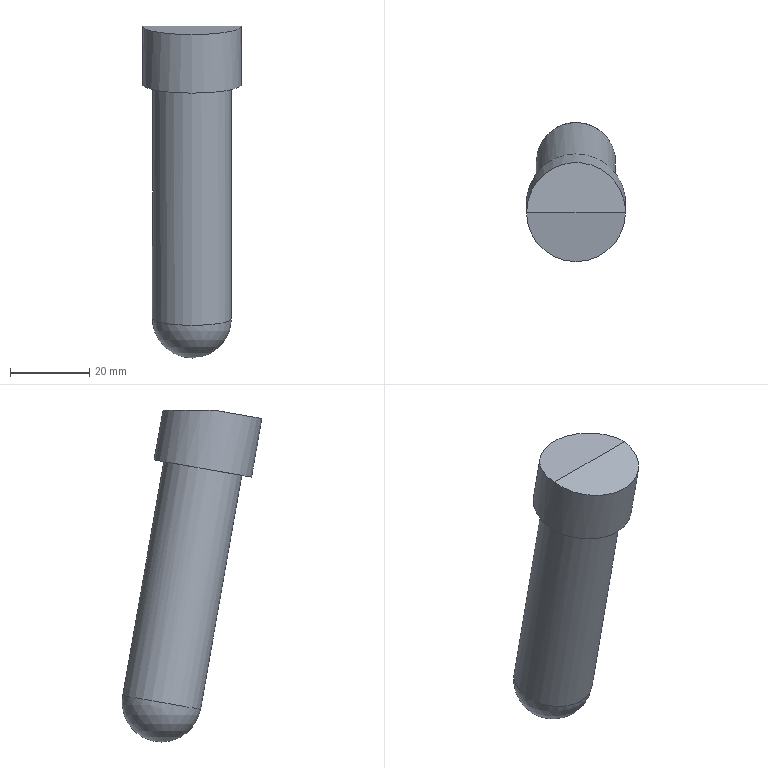Part | STEP file | P011002S001-008 | 1 solid | 6 faces | box 25 x 35.334 x 83.861 mm | volume 28077 mm3 | plane 3 | cylinder 2 | sphere 1 | commonest cylinder face diameters 20 x1 25 x1
STEP:
#1=CARTESIAN_POINT('',(0.,0.,0.));
#2=DIRECTION('',(0.,0.,1.));
#3=DIRECTION('',(1.,0.,0.));
#4=AXIS2_PLACEMENT_3D('',#1,#2,#3);
#5=CARTESIAN_POINT('',(12.,220.,76.));
#6=VERTEX_POINT('',#5);
#7=CARTESIAN_POINT('',(-0.5,207.69,73.829));
#8=VERTEX_POINT('',#7);
#9=CARTESIAN_POINT('',(-0.5,220.,76.));
#10=DIRECTION('',(0.,0.1736,-0.9848));
#11=DIRECTION('',(0.,-0.9848,-0.1736));
#12=AXIS2_PLACEMENT_3D('',#9,#10,#11);
#13=CIRCLE('',#12,12.5);
#14=CARTESIAN_POINT('',(-0.5,220.,76.));
#15=DIRECTION('',(0.,-0.1736,0.9848));
#16=DIRECTION('',(0.,-0.9848,-0.1736));
#17=AXIS2_PLACEMENT_3D('',#14,#15,#16);
#18=PLANE('',#17);
#19=CARTESIAN_POINT('',(12.5,0.));
#20=CARTESIAN_POINT('',(12.5,-21.651));
#21=CARTESIAN_POINT('',(-6.25,-10.825));
#22=CARTESIAN_POINT('',(-25.,0.));
#23=CARTESIAN_POINT('',(-6.25,10.825));
#24=CARTESIAN_POINT('',(12.5,21.651));
#25=CARTESIAN_POINT('',(12.5,0.));
#26=(BOUNDED_CURVE()B_SPLINE_CURVE(2,(#19,#20,#21,#22,#23,#24,#25),.UNSPECIFIED.,.T.,.F.)B_SPLINE_CURVE_WITH_KNOTS((1,2,2,2,2,1),(-2.094,0.,2.094,4.189,6.283,8.378),.UNSPECIFIED.)CURVE()GEOMETRIC_REPRESENTATION_ITEM()RATIONAL_B_SPLINE_CURVE((1.,0.5,1.,0.5,1.,0.5,1.))REPRESENTATION_ITEM(''));
#27=(GEOMETRIC_REPRESENTATION_CONTEXT(2)PARAMETRIC_REPRESENTATION_CONTEXT()REPRESENTATION_CONTEXT('',''));
#28=DEFINITIONAL_REPRESENTATION('',(#26),#27);
#29=PCURVE('',#18,#28);
#30=CARTESIAN_POINT('',(-0.5,254.647,-120.494));
#31=DIRECTION('',(0.,-0.1736,0.9848));
#32=DIRECTION('',(0.,-0.9848,-0.1736));
#33=AXIS2_PLACEMENT_3D('',#30,#31,#32);
#34=CYLINDRICAL_SURFACE('',#33,12.5);
#35=CARTESIAN_POINT('',(6.283,199.525));
#36=DIRECTION('',(-1.,0.));
#37=VECTOR('',#36,1.);
#38=LINE('',#35,#37);
#39=(GEOMETRIC_REPRESENTATION_CONTEXT(2)PARAMETRIC_REPRESENTATION_CONTEXT()REPRESENTATION_CONTEXT('',''));
#40=DEFINITIONAL_REPRESENTATION('',(#38),#39);
#41=PCURVE('',#34,#40);
#42=SURFACE_CURVE('',#13,(#29,#41),.PCURVE_S1.);
#43=EDGE_CURVE('',#6,#8,#42,.T.);
#44=ORIENTED_EDGE('',*,*,#43,.F.);
#45=CARTESIAN_POINT('',(-13.,220.,76.));
#46=VERTEX_POINT('',#45);
#47=CARTESIAN_POINT('',(-0.5,220.,76.));
#48=DIRECTION('',(1.,0.,0.));
#49=VECTOR('',#48,1.);
#50=LINE('',#47,#49);
#51=CARTESIAN_POINT('',(0.,0.));
#52=DIRECTION('',(0.,1.));
#53=VECTOR('',#52,1.);
#54=LINE('',#51,#53);
#55=(GEOMETRIC_REPRESENTATION_CONTEXT(2)PARAMETRIC_REPRESENTATION_CONTEXT()REPRESENTATION_CONTEXT('',''));
#56=DEFINITIONAL_REPRESENTATION('',(#54),#55);
#57=PCURVE('',#18,#56);
#58=CARTESIAN_POINT('',(49.5,200.,76.));
#59=DIRECTION('',(0.,0.,1.));
#60=DIRECTION('',(-1.,0.,0.));
#61=AXIS2_PLACEMENT_3D('',#58,#59,#60);
#62=PLANE('',#61);
#63=CARTESIAN_POINT('',(50.,-20.));
#64=DIRECTION('',(-1.,0.));
#65=VECTOR('',#64,1.);
#66=LINE('',#63,#65);
#67=(GEOMETRIC_REPRESENTATION_CONTEXT(2)PARAMETRIC_REPRESENTATION_CONTEXT()REPRESENTATION_CONTEXT('',''));
#68=DEFINITIONAL_REPRESENTATION('',(#66),#67);
#69=PCURVE('',#62,#68);
#70=SURFACE_CURVE('',#50,(#57,#69),.PCURVE_S1.);
#71=EDGE_CURVE('',#46,#6,#70,.T.);
#72=ORIENTED_EDGE('',*,*,#71,.F.);
#73=CARTESIAN_POINT('',(-0.5,220.,76.));
#74=DIRECTION('',(0.,0.1736,-0.9848));
#75=DIRECTION('',(0.,-0.9848,-0.1736));
#76=AXIS2_PLACEMENT_3D('',#73,#74,#75);
#77=CIRCLE('',#76,12.5);
#78=CARTESIAN_POINT('',(12.5,0.));
#79=CARTESIAN_POINT('',(12.5,-21.651));
#80=CARTESIAN_POINT('',(-6.25,-10.825));
#81=CARTESIAN_POINT('',(-25.,0.));
#82=CARTESIAN_POINT('',(-6.25,10.825));
#83=CARTESIAN_POINT('',(12.5,21.651));
#84=CARTESIAN_POINT('',(12.5,0.));
#85=(BOUNDED_CURVE()B_SPLINE_CURVE(2,(#78,#79,#80,#81,#82,#83,#84),.UNSPECIFIED.,.T.,.F.)B_SPLINE_CURVE_WITH_KNOTS((1,2,2,2,2,1),(-2.094,0.,2.094,4.189,6.283,8.378),.UNSPECIFIED.)CURVE()GEOMETRIC_REPRESENTATION_ITEM()RATIONAL_B_SPLINE_CURVE((1.,0.5,1.,0.5,1.,0.5,1.))REPRESENTATION_ITEM(''));
#86=(GEOMETRIC_REPRESENTATION_CONTEXT(2)PARAMETRIC_REPRESENTATION_CONTEXT()REPRESENTATION_CONTEXT('',''));
#87=DEFINITIONAL_REPRESENTATION('',(#85),#86);
#88=PCURVE('',#18,#87);
#89=CARTESIAN_POINT('',(12.566,199.525));
#90=DIRECTION('',(-1.,0.));
#91=VECTOR('',#90,1.);
#92=LINE('',#89,#91);
#93=(GEOMETRIC_REPRESENTATION_CONTEXT(2)PARAMETRIC_REPRESENTATION_CONTEXT()REPRESENTATION_CONTEXT('',''));
#94=DEFINITIONAL_REPRESENTATION('',(#92),#93);
#95=PCURVE('',#34,#94);
#96=SURFACE_CURVE('',#77,(#88,#95),.PCURVE_S1.);
#97=EDGE_CURVE('',#8,#46,#96,.T.);
#98=ORIENTED_EDGE('',*,*,#97,.F.);
#99=EDGE_LOOP('',(#44,#72,#98));
#100=FACE_BOUND('',#99,.T.);
#101=ADVANCED_FACE('',(#100),#18,.T.);
#102=CARTESIAN_POINT('',(-0.5,210.295,59.057));
#103=VERTEX_POINT('',#102);
#104=CARTESIAN_POINT('',(-0.5,222.605,61.228));
#105=DIRECTION('',(0.,0.1736,-0.9848));
#106=DIRECTION('',(0.,-0.9848,-0.1736));
#107=AXIS2_PLACEMENT_3D('',#104,#105,#106);
#108=CIRCLE('',#107,12.5);
#109=CARTESIAN_POINT('',(6.283,184.525));
#110=DIRECTION('',(-1.,0.));
#111=VECTOR('',#110,1.);
#112=LINE('',#109,#111);
#113=(GEOMETRIC_REPRESENTATION_CONTEXT(2)PARAMETRIC_REPRESENTATION_CONTEXT()REPRESENTATION_CONTEXT('',''));
#114=DEFINITIONAL_REPRESENTATION('',(#112),#113);
#115=PCURVE('',#34,#114);
#116=CARTESIAN_POINT('',(-0.5,222.605,61.228));
#117=DIRECTION('',(0.,-0.1736,0.9848));
#118=DIRECTION('',(0.,-0.9848,-0.1736));
#119=AXIS2_PLACEMENT_3D('',#116,#117,#118);
#120=PLANE('',#119);
#121=CARTESIAN_POINT('',(12.5,0.));
#122=CARTESIAN_POINT('',(12.5,-21.651));
#123=CARTESIAN_POINT('',(-6.25,-10.825));
#124=CARTESIAN_POINT('',(-25.,0.));
#125=CARTESIAN_POINT('',(-6.25,10.825));
#126=CARTESIAN_POINT('',(12.5,21.651));
#127=CARTESIAN_POINT('',(12.5,0.));
#128=(BOUNDED_CURVE()B_SPLINE_CURVE(2,(#121,#122,#123,#124,#125,#126,#127),.UNSPECIFIED.,.T.,.F.)B_SPLINE_CURVE_WITH_KNOTS((1,2,2,2,2,1),(-2.094,0.,2.094,4.189,6.283,8.378),.UNSPECIFIED.)CURVE()GEOMETRIC_REPRESENTATION_ITEM()RATIONAL_B_SPLINE_CURVE((1.,0.5,1.,0.5,1.,0.5,1.))REPRESENTATION_ITEM(''));
#129=(GEOMETRIC_REPRESENTATION_CONTEXT(2)PARAMETRIC_REPRESENTATION_CONTEXT()REPRESENTATION_CONTEXT('',''));
#130=DEFINITIONAL_REPRESENTATION('',(#128),#129);
#131=PCURVE('',#120,#130);
#132=SURFACE_CURVE('',#108,(#115,#131),.PCURVE_S1.);
#133=EDGE_CURVE('',#103,#103,#132,.T.);
#134=ORIENTED_EDGE('',*,*,#133,.F.);
#135=CARTESIAN_POINT('',(-0.5,210.295,59.057));
#136=CARTESIAN_POINT('',(-0.5,207.69,73.829));
#137=B_SPLINE_CURVE_WITH_KNOTS('',1,(#135,#136),.UNSPECIFIED.,.F.,.F.,(2,2),(184.525,199.525),.PIECEWISE_BEZIER_KNOTS.);
#138=CARTESIAN_POINT('',(6.283,0.));
#139=DIRECTION('',(0.,1.));
#140=VECTOR('',#139,1.);
#141=LINE('',#138,#140);
#142=(GEOMETRIC_REPRESENTATION_CONTEXT(2)PARAMETRIC_REPRESENTATION_CONTEXT()REPRESENTATION_CONTEXT('',''));
#143=DEFINITIONAL_REPRESENTATION('',(#141),#142);
#144=PCURVE('',#34,#143);
#145=CARTESIAN_POINT('',(0.,0.));
#146=DIRECTION('',(0.,1.));
#147=VECTOR('',#146,1.);
#148=LINE('',#145,#147);
#149=(GEOMETRIC_REPRESENTATION_CONTEXT(2)PARAMETRIC_REPRESENTATION_CONTEXT()REPRESENTATION_CONTEXT('',''));
#150=DEFINITIONAL_REPRESENTATION('',(#148),#149);
#151=PCURVE('',#34,#150);
#152=SEAM_CURVE('',#137,(#144,#151),.PCURVE_S1.);
#153=EDGE_CURVE('',#103,#8,#152,.T.);
#154=ORIENTED_EDGE('',*,*,#153,.T.);
#155=ORIENTED_EDGE('',*,*,#97,.T.);
#156=CARTESIAN_POINT('',(-0.5,220.,76.));
#157=DIRECTION('',(0.,0.,-1.));
#158=DIRECTION('',(0.,-1.,0.));
#159=AXIS2_PLACEMENT_3D('',#156,#157,#158);
#160=ELLIPSE('',#159,12.693,12.5);
#161=CARTESIAN_POINT('',(4.712,199.525));
#162=CARTESIAN_POINT('',(4.665,199.421));
#163=CARTESIAN_POINT('',(4.57,199.211));
#164=CARTESIAN_POINT('',(4.427,198.902));
#165=CARTESIAN_POINT('',(4.284,198.607));
#166=CARTESIAN_POINT('',(4.141,198.33));
#167=CARTESIAN_POINT('',(3.998,198.077));
#168=CARTESIAN_POINT('',(3.856,197.854));
#169=CARTESIAN_POINT('',(3.713,197.665));
#170=CARTESIAN_POINT('',(3.57,197.514));
#171=CARTESIAN_POINT('',(3.427,197.403));
#172=CARTESIAN_POINT('',(3.284,197.336));
#173=CARTESIAN_POINT('',(3.142,197.314));
#174=CARTESIAN_POINT('',(2.999,197.336));
#175=CARTESIAN_POINT('',(2.856,197.403));
#176=CARTESIAN_POINT('',(2.713,197.514));
#177=CARTESIAN_POINT('',(2.57,197.665));
#178=CARTESIAN_POINT('',(2.428,197.854));
#179=CARTESIAN_POINT('',(2.285,198.077));
#180=CARTESIAN_POINT('',(2.142,198.33));
#181=CARTESIAN_POINT('',(1.999,198.607));
#182=CARTESIAN_POINT('',(1.856,198.902));
#183=CARTESIAN_POINT('',(1.714,199.211));
#184=CARTESIAN_POINT('',(1.618,199.421));
#185=CARTESIAN_POINT('',(1.571,199.525));
#186=B_SPLINE_CURVE_WITH_KNOTS('',3,(#161,#162,#163,#164,#165,#166,#167,#168,#169,#170,#171,#172,#173,#174,#175,#176,#177,#178,#179,#180,#181,#182,#183,#184,#185),.UNSPECIFIED.,.F.,.F.,(4,1,1,1,1,1,1,1,1,1,1,1,1,1,1,1,1,1,1,1,1,1,4),(1.571,1.714,1.856,1.999,2.142,2.285,2.428,2.57,2.713,2.856,2.999,3.142,3.284,3.427,3.57,3.713,3.856,3.998,4.141,4.284,4.427,4.57,4.712),.QUASI_UNIFORM_KNOTS.);
#187=(GEOMETRIC_REPRESENTATION_CONTEXT(2)PARAMETRIC_REPRESENTATION_CONTEXT()REPRESENTATION_CONTEXT('',''));
#188=DEFINITIONAL_REPRESENTATION('',(#186),#187);
#189=PCURVE('',#34,#188);
#190=CARTESIAN_POINT('',(50.,-7.307));
#191=CARTESIAN_POINT('',(71.651,-7.307));
#192=CARTESIAN_POINT('',(60.825,-26.346));
#193=CARTESIAN_POINT('',(50.,-45.386));
#194=CARTESIAN_POINT('',(39.175,-26.346));
#195=CARTESIAN_POINT('',(28.349,-7.307));
#196=CARTESIAN_POINT('',(50.,-7.307));
#197=(BOUNDED_CURVE()B_SPLINE_CURVE(2,(#190,#191,#192,#193,#194,#195,#196),.UNSPECIFIED.,.T.,.F.)B_SPLINE_CURVE_WITH_KNOTS((1,2,2,2,2,1),(-2.094,0.,2.094,4.189,6.283,8.378),.UNSPECIFIED.)CURVE()GEOMETRIC_REPRESENTATION_ITEM()RATIONAL_B_SPLINE_CURVE((1.,0.5,1.,0.5,1.,0.5,1.))REPRESENTATION_ITEM(''));
#198=(GEOMETRIC_REPRESENTATION_CONTEXT(2)PARAMETRIC_REPRESENTATION_CONTEXT()REPRESENTATION_CONTEXT('',''));
#199=DEFINITIONAL_REPRESENTATION('',(#197),#198);
#200=PCURVE('',#62,#199);
#201=SURFACE_CURVE('',#160,(#189,#200),.PCURVE_S1.);
#202=EDGE_CURVE('',#46,#6,#201,.T.);
#203=ORIENTED_EDGE('',*,*,#202,.T.);
#204=ORIENTED_EDGE('',*,*,#43,.T.);
#205=ORIENTED_EDGE('',*,*,#153,.F.);
#206=EDGE_LOOP('',(#134,#154,#155,#203,#204,#205));
#207=FACE_BOUND('',#206,.T.);
#208=ADVANCED_FACE('',(#207),#34,.T.);
#209=CARTESIAN_POINT('',(-0.5,223.176,0.4029));
#210=VERTEX_POINT('',#209);
#211=CARTESIAN_POINT('',(-10.5,233.024,2.139));
#212=VERTEX_POINT('',#211);
#213=CARTESIAN_POINT('',(-0.5,233.024,2.139));
#214=DIRECTION('',(0.,0.1736,-0.9848));
#215=DIRECTION('',(0.,-0.9848,-0.1736));
#216=AXIS2_PLACEMENT_3D('',#213,#214,#215);
#217=CIRCLE('',#216,10.);
#218=CARTESIAN_POINT('',(-0.5,254.647,-120.494));
#219=DIRECTION('',(0.,-0.1736,0.9848));
#220=DIRECTION('',(0.,-0.9848,-0.1736));
#221=AXIS2_PLACEMENT_3D('',#218,#219,#220);
#222=CYLINDRICAL_SURFACE('',#221,10.);
#223=CARTESIAN_POINT('',(6.283,124.525));
#224=DIRECTION('',(-1.,0.));
#225=VECTOR('',#224,1.);
#226=LINE('',#223,#225);
#227=(GEOMETRIC_REPRESENTATION_CONTEXT(2)PARAMETRIC_REPRESENTATION_CONTEXT()REPRESENTATION_CONTEXT('',''));
#228=DEFINITIONAL_REPRESENTATION('',(#226),#227);
#229=PCURVE('',#222,#228);
#230=CARTESIAN_POINT('',(-0.5,233.024,2.139));
#231=DIRECTION('',(0.,0.,1.));
#232=DIRECTION('',(-1.,0.,0.));
#233=AXIS2_PLACEMENT_3D('',#230,#231,#232);
#234=SPHERICAL_SURFACE('',#233,10.);
#235=CARTESIAN_POINT('',(1.571,-0.1745));
#236=CARTESIAN_POINT('',(1.474,-0.1746));
#237=CARTESIAN_POINT('',(1.281,-0.1697));
#238=CARTESIAN_POINT('',(0.9922,-0.1486));
#239=CARTESIAN_POINT('',(0.706,-0.1155));
#240=CARTESIAN_POINT('',(0.4223,-0.07316));
#241=CARTESIAN_POINT('',(0.1405,-0.02504));
#242=CARTESIAN_POINT('',(-0.1405,0.02504));
#243=CARTESIAN_POINT('',(-0.4223,0.07316));
#244=CARTESIAN_POINT('',(-0.706,0.1155));
#245=CARTESIAN_POINT('',(-0.9922,0.1486));
#246=CARTESIAN_POINT('',(-1.281,0.1697));
#247=CARTESIAN_POINT('',(-1.571,0.1769));
#248=CARTESIAN_POINT('',(-1.861,0.1697));
#249=CARTESIAN_POINT('',(-2.149,0.1486));
#250=CARTESIAN_POINT('',(-2.436,0.1155));
#251=CARTESIAN_POINT('',(-2.719,0.07316));
#252=CARTESIAN_POINT('',(-3.001,0.02504));
#253=CARTESIAN_POINT('',(-3.282,-0.02504));
#254=CARTESIAN_POINT('',(-3.564,-0.07316));
#255=CARTESIAN_POINT('',(-3.848,-0.1155));
#256=CARTESIAN_POINT('',(-4.134,-0.1486));
#257=CARTESIAN_POINT('',(-4.422,-0.1697));
#258=CARTESIAN_POINT('',(-4.616,-0.1746));
#259=CARTESIAN_POINT('',(-4.712,-0.1745));
#260=B_SPLINE_CURVE_WITH_KNOTS('',3,(#235,#236,#237,#238,#239,#240,#241,#242,#243,#244,#245,#246,#247,#248,#249,#250,#251,#252,#253,#254,#255,#256,#257,#258,#259),.UNSPECIFIED.,.F.,.F.,(4,1,1,1,1,1,1,1,1,1,1,1,1,1,1,1,1,1,1,1,1,1,4),(0.,0.2856,0.5712,0.8568,1.142,1.428,1.714,1.999,2.285,2.57,2.856,3.142,3.427,3.713,3.998,4.284,4.57,4.855,5.141,5.426,5.712,5.998,6.283),.QUASI_UNIFORM_KNOTS.);
#261=(GEOMETRIC_REPRESENTATION_CONTEXT(2)PARAMETRIC_REPRESENTATION_CONTEXT()REPRESENTATION_CONTEXT('',''));
#262=DEFINITIONAL_REPRESENTATION('',(#260),#261);
#263=PCURVE('',#234,#262);
#264=SURFACE_CURVE('',#217,(#229,#263),.PCURVE_S1.);
#265=EDGE_CURVE('',#210,#212,#264,.T.);
#266=ORIENTED_EDGE('',*,*,#265,.F.);
#267=CARTESIAN_POINT('',(-0.5,212.757,59.491));
#268=VERTEX_POINT('',#267);
#269=CARTESIAN_POINT('',(-0.5,223.176,0.4029));
#270=CARTESIAN_POINT('',(-0.5,212.757,59.491));
#271=B_SPLINE_CURVE_WITH_KNOTS('',1,(#269,#270),.UNSPECIFIED.,.F.,.F.,(2,2),(124.525,184.525),.PIECEWISE_BEZIER_KNOTS.);
#272=CARTESIAN_POINT('',(6.283,0.));
#273=DIRECTION('',(0.,1.));
#274=VECTOR('',#273,1.);
#275=LINE('',#272,#274);
#276=(GEOMETRIC_REPRESENTATION_CONTEXT(2)PARAMETRIC_REPRESENTATION_CONTEXT()REPRESENTATION_CONTEXT('',''));
#277=DEFINITIONAL_REPRESENTATION('',(#275),#276);
#278=PCURVE('',#222,#277);
#279=CARTESIAN_POINT('',(0.,0.));
#280=DIRECTION('',(0.,1.));
#281=VECTOR('',#280,1.);
#282=LINE('',#279,#281);
#283=(GEOMETRIC_REPRESENTATION_CONTEXT(2)PARAMETRIC_REPRESENTATION_CONTEXT()REPRESENTATION_CONTEXT('',''));
#284=DEFINITIONAL_REPRESENTATION('',(#282),#283);
#285=PCURVE('',#222,#284);
#286=SEAM_CURVE('',#271,(#278,#285),.PCURVE_S1.);
#287=EDGE_CURVE('',#210,#268,#286,.T.);
#288=ORIENTED_EDGE('',*,*,#287,.T.);
#289=CARTESIAN_POINT('',(-0.5,222.605,61.228));
#290=DIRECTION('',(0.,0.1736,-0.9848));
#291=DIRECTION('',(0.,-0.9848,-0.1736));
#292=AXIS2_PLACEMENT_3D('',#289,#290,#291);
#293=CIRCLE('',#292,10.);
#294=CARTESIAN_POINT('',(6.283,184.525));
#295=DIRECTION('',(-1.,0.));
#296=VECTOR('',#295,1.);
#297=LINE('',#294,#296);
#298=(GEOMETRIC_REPRESENTATION_CONTEXT(2)PARAMETRIC_REPRESENTATION_CONTEXT()REPRESENTATION_CONTEXT('',''));
#299=DEFINITIONAL_REPRESENTATION('',(#297),#298);
#300=PCURVE('',#222,#299);
#301=CARTESIAN_POINT('',(10.,0.));
#302=CARTESIAN_POINT('',(10.,-17.321));
#303=CARTESIAN_POINT('',(-5.,-8.66));
#304=CARTESIAN_POINT('',(-20.,0.));
#305=CARTESIAN_POINT('',(-5.,8.66));
#306=CARTESIAN_POINT('',(10.,17.321));
#307=CARTESIAN_POINT('',(10.,0.));
#308=(BOUNDED_CURVE()B_SPLINE_CURVE(2,(#301,#302,#303,#304,#305,#306,#307),.UNSPECIFIED.,.T.,.F.)B_SPLINE_CURVE_WITH_KNOTS((1,2,2,2,2,1),(-2.094,0.,2.094,4.189,6.283,8.378),.UNSPECIFIED.)CURVE()GEOMETRIC_REPRESENTATION_ITEM()RATIONAL_B_SPLINE_CURVE((1.,0.5,1.,0.5,1.,0.5,1.))REPRESENTATION_ITEM(''));
#309=(GEOMETRIC_REPRESENTATION_CONTEXT(2)PARAMETRIC_REPRESENTATION_CONTEXT()REPRESENTATION_CONTEXT('',''));
#310=DEFINITIONAL_REPRESENTATION('',(#308),#309);
#311=PCURVE('',#120,#310);
#312=SURFACE_CURVE('',#293,(#300,#311),.PCURVE_S1.);
#313=EDGE_CURVE('',#268,#268,#312,.T.);
#314=ORIENTED_EDGE('',*,*,#313,.T.);
#315=ORIENTED_EDGE('',*,*,#287,.F.);
#316=CARTESIAN_POINT('',(-0.5,233.024,2.139));
#317=DIRECTION('',(0.,0.1736,-0.9848));
#318=DIRECTION('',(0.,-0.9848,-0.1736));
#319=AXIS2_PLACEMENT_3D('',#316,#317,#318);
#320=CIRCLE('',#319,10.);
#321=CARTESIAN_POINT('',(6.283,124.525));
#322=DIRECTION('',(-1.,0.));
#323=VECTOR('',#322,1.);
#324=LINE('',#321,#323);
#325=(GEOMETRIC_REPRESENTATION_CONTEXT(2)PARAMETRIC_REPRESENTATION_CONTEXT()REPRESENTATION_CONTEXT('',''));
#326=DEFINITIONAL_REPRESENTATION('',(#324),#325);
#327=PCURVE('',#222,#326);
#328=CARTESIAN_POINT('',(7.854,-0.1745));
#329=CARTESIAN_POINT('',(7.757,-0.1746));
#330=CARTESIAN_POINT('',(7.564,-0.1697));
#331=CARTESIAN_POINT('',(7.275,-0.1486));
#332=CARTESIAN_POINT('',(6.989,-0.1155));
#333=CARTESIAN_POINT('',(6.706,-0.07316));
#334=CARTESIAN_POINT('',(6.424,-0.02504));
#335=CARTESIAN_POINT('',(6.143,0.02504));
#336=CARTESIAN_POINT('',(5.861,0.07316));
#337=CARTESIAN_POINT('',(5.577,0.1155));
#338=CARTESIAN_POINT('',(5.291,0.1486));
#339=CARTESIAN_POINT('',(5.002,0.1697));
#340=CARTESIAN_POINT('',(4.712,0.1769));
#341=CARTESIAN_POINT('',(4.422,0.1697));
#342=CARTESIAN_POINT('',(4.134,0.1486));
#343=CARTESIAN_POINT('',(3.848,0.1155));
#344=CARTESIAN_POINT('',(3.564,0.07316));
#345=CARTESIAN_POINT('',(3.282,0.02504));
#346=CARTESIAN_POINT('',(3.001,-0.02504));
#347=CARTESIAN_POINT('',(2.719,-0.07316));
#348=CARTESIAN_POINT('',(2.436,-0.1155));
#349=CARTESIAN_POINT('',(2.149,-0.1486));
#350=CARTESIAN_POINT('',(1.861,-0.1697));
#351=CARTESIAN_POINT('',(1.668,-0.1746));
#352=CARTESIAN_POINT('',(1.571,-0.1745));
#353=B_SPLINE_CURVE_WITH_KNOTS('',3,(#328,#329,#330,#331,#332,#333,#334,#335,#336,#337,#338,#339,#340,#341,#342,#343,#344,#345,#346,#347,#348,#349,#350,#351,#352),.UNSPECIFIED.,.F.,.F.,(4,1,1,1,1,1,1,1,1,1,1,1,1,1,1,1,1,1,1,1,1,1,4),(0.,0.2856,0.5712,0.8568,1.142,1.428,1.714,1.999,2.285,2.57,2.856,3.142,3.427,3.713,3.998,4.284,4.57,4.855,5.141,5.426,5.712,5.998,6.283),.QUASI_UNIFORM_KNOTS.);
#354=(GEOMETRIC_REPRESENTATION_CONTEXT(2)PARAMETRIC_REPRESENTATION_CONTEXT()REPRESENTATION_CONTEXT('',''));
#355=DEFINITIONAL_REPRESENTATION('',(#353),#354);
#356=PCURVE('',#234,#355);
#357=SURFACE_CURVE('',#320,(#327,#356),.PCURVE_S1.);
#358=EDGE_CURVE('',#212,#210,#357,.T.);
#359=ORIENTED_EDGE('',*,*,#358,.F.);
#360=EDGE_LOOP('',(#266,#288,#314,#315,#359));
#361=FACE_BOUND('',#360,.T.);
#362=ADVANCED_FACE('',(#361),#222,.T.);
#363=ORIENTED_EDGE('',*,*,#133,.T.);
#364=EDGE_LOOP('',(#363));
#365=FACE_BOUND('',#364,.T.);
#366=ORIENTED_EDGE('',*,*,#313,.F.);
#367=EDGE_LOOP('',(#366));
#368=FACE_BOUND('',#367,.T.);
#369=ADVANCED_FACE('',(#365,#368),#120,.F.);
#370=ORIENTED_EDGE('',*,*,#265,.T.);
#371=CARTESIAN_POINT('',(-0.5,233.024,-7.861));
#372=VERTEX_POINT('',#371);
#373=CARTESIAN_POINT('',(-0.5,233.024,-7.861));
#374=CARTESIAN_POINT('',(-2.744,233.024,-7.861));
#375=CARTESIAN_POINT('',(-4.988,233.024,-7.273));
#376=CARTESIAN_POINT('',(-7.047,233.024,-6.098));
#377=CARTESIAN_POINT('',(-8.738,233.024,-4.408));
#378=CARTESIAN_POINT('',(-9.913,233.024,-2.349));
#379=CARTESIAN_POINT('',(-10.5,233.024,-0.1046));
#380=CARTESIAN_POINT('',(-10.5,233.024,2.139));
#381=B_SPLINE_CURVE_WITH_KNOTS('',7,(#373,#374,#375,#376,#377,#378,#379,#380),.UNSPECIFIED.,.F.,.F.,(8,8),(-1.571,0.000000068),.PIECEWISE_BEZIER_KNOTS.);
#382=CARTESIAN_POINT('',(0.,0.));
#383=DIRECTION('',(0.,1.));
#384=VECTOR('',#383,1.);
#385=LINE('',#382,#384);
#386=(GEOMETRIC_REPRESENTATION_CONTEXT(2)PARAMETRIC_REPRESENTATION_CONTEXT()REPRESENTATION_CONTEXT('',''));
#387=DEFINITIONAL_REPRESENTATION('',(#385),#386);
#388=PCURVE('',#234,#387);
#389=CARTESIAN_POINT('',(6.283,0.));
#390=DIRECTION('',(0.,1.));
#391=VECTOR('',#390,1.);
#392=LINE('',#389,#391);
#393=(GEOMETRIC_REPRESENTATION_CONTEXT(2)PARAMETRIC_REPRESENTATION_CONTEXT()REPRESENTATION_CONTEXT('',''));
#394=DEFINITIONAL_REPRESENTATION('',(#392),#393);
#395=PCURVE('',#234,#394);
#396=SEAM_CURVE('',#381,(#388,#395),.PCURVE_S1.);
#397=EDGE_CURVE('',#372,#212,#396,.T.);
#398=ORIENTED_EDGE('',*,*,#397,.F.);
#399=ORIENTED_EDGE('',*,*,#397,.T.);
#400=ORIENTED_EDGE('',*,*,#358,.T.);
#401=EDGE_LOOP('',(#370,#398,#399,#400));
#402=FACE_BOUND('',#401,.T.);
#403=ADVANCED_FACE('',(#402),#234,.T.);
#404=ORIENTED_EDGE('',*,*,#71,.T.);
#405=ORIENTED_EDGE('',*,*,#202,.F.);
#406=EDGE_LOOP('',(#404,#405));
#407=FACE_BOUND('',#406,.T.);
#408=ADVANCED_FACE('',(#407),#62,.T.);
#409=CLOSED_SHELL('',(#101,#208,#362,#369,#403,#408));
#410=MANIFOLD_SOLID_BREP('',#409);
#411=(LENGTH_UNIT()NAMED_UNIT(*)SI_UNIT(.MILLI.,.METRE.));
#412=UNCERTAINTY_MEASURE_WITH_UNIT(LENGTH_MEASURE(0.0001),#411,'','');
#413=(NAMED_UNIT(*)PLANE_ANGLE_UNIT()SI_UNIT($,.RADIAN.));
#414=(NAMED_UNIT(*)SI_UNIT($,.STERADIAN.)SOLID_ANGLE_UNIT());
#415=(GEOMETRIC_REPRESENTATION_CONTEXT(3)GLOBAL_UNCERTAINTY_ASSIGNED_CONTEXT((#412))GLOBAL_UNIT_ASSIGNED_CONTEXT((#411,#413,#414))REPRESENTATION_CONTEXT('',''));
#416=ADVANCED_BREP_SHAPE_REPRESENTATION('',(#4,#410),#415);